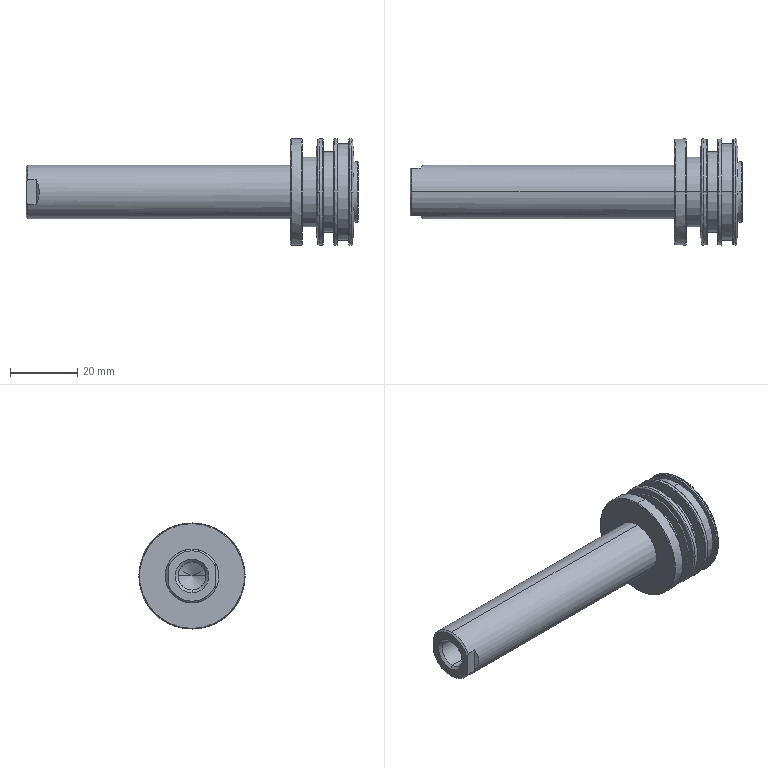Part | STEP file | TR_32x10-4 | 1 solid | 65 faces | box 98.8 x 31.6 x 31.6 mm | volume 26490 mm3 | cone 25 | cylinder 20 | plane 16 | spline 4 | commonest cylinder face diameters 31.6 x8 8.376 x2 16 x2 18 x2 20.8 x2 24 x2